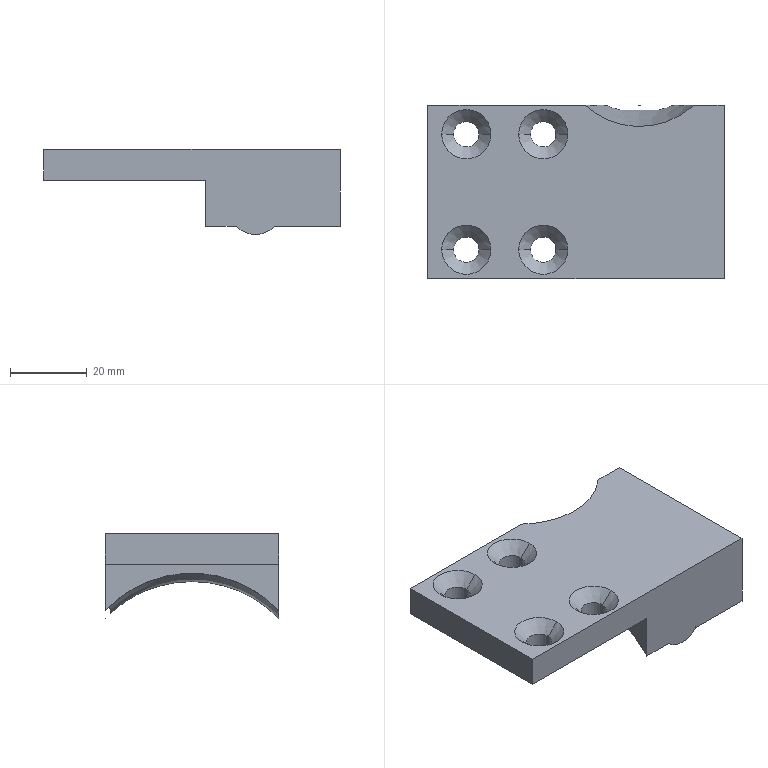Part | STEP file | PTFE block (lower) | 2 solids | 33 faces | box 77 x 45 x 22.101 mm | volume 33979 mm3 | plane 12 | cylinder 10 | cone 8 | spline 3 | commonest cylinder face diameters 6.6 x8 62 x2